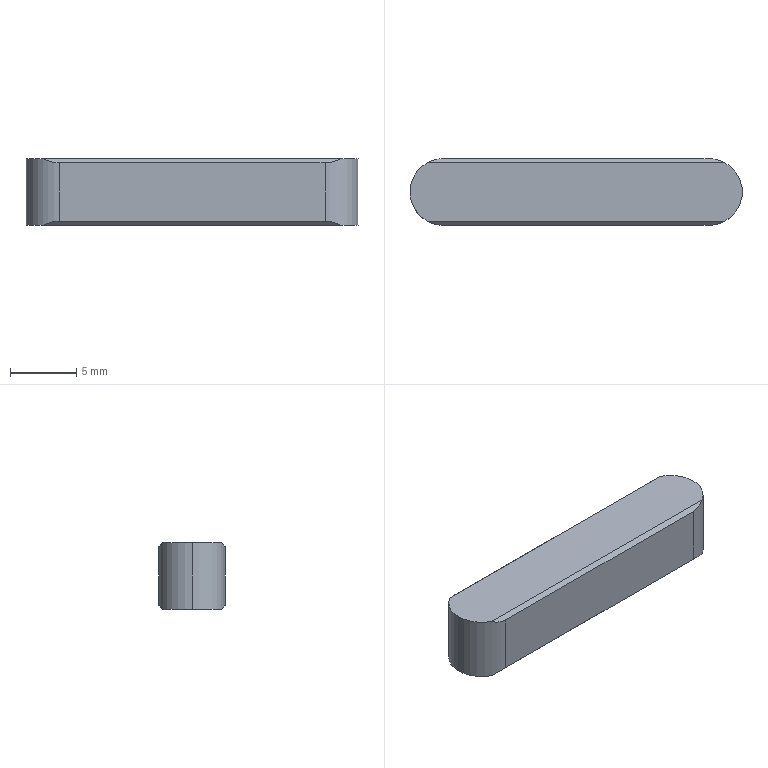Part | STEP file | 0228_010_KES5-25 | 1 solid | 11 faces | box 25 x 5 x 5 mm | volume 594.343 mm3 | plane 8 | cylinder 3 | commonest cylinder face diameters 5 x3
STEP:
#1=CARTESIAN_POINT('',(0.,0.,0.));
#2=DIRECTION('',(0.,0.,1.));
#3=DIRECTION('',(1.,0.,0.));
#4=AXIS2_PLACEMENT_3D('',#1,#2,#3);
#5=CARTESIAN_POINT('',(1.313,0.3,5.));
#6=VERTEX_POINT('',#5);
#7=CARTESIAN_POINT('',(0.,2.5,5.));
#8=VERTEX_POINT('',#7);
#9=CARTESIAN_POINT('',(2.5,2.5,5.));
#10=DIRECTION('',(0.,0.,-1.));
#11=DIRECTION('',(-1.,0.,0.));
#12=AXIS2_PLACEMENT_3D('',#9,#10,#11);
#13=CIRCLE('',#12,2.5);
#14=CARTESIAN_POINT('',(2.5,2.5,0.));
#15=DIRECTION('',(0.,0.,-1.));
#16=DIRECTION('',(-1.,0.,0.));
#17=AXIS2_PLACEMENT_3D('',#14,#15,#16);
#18=CYLINDRICAL_SURFACE('',#17,2.5);
#19=CARTESIAN_POINT('',(0.,-5.));
#20=DIRECTION('',(1.,0.));
#21=VECTOR('',#20,1.);
#22=LINE('',#19,#21);
#23=(GEOMETRIC_REPRESENTATION_CONTEXT(2)PARAMETRIC_REPRESENTATION_CONTEXT()REPRESENTATION_CONTEXT('',''));
#24=DEFINITIONAL_REPRESENTATION('',(#22),#23);
#25=PCURVE('',#18,#24);
#26=CARTESIAN_POINT('',(0.,0.,5.));
#27=DIRECTION('',(0.,0.,1.));
#28=DIRECTION('',(1.,0.,0.));
#29=AXIS2_PLACEMENT_3D('',#26,#27,#28);
#30=PLANE('',#29);
#31=CARTESIAN_POINT('',(0.,2.5));
#32=CARTESIAN_POINT('',(0.,6.83));
#33=CARTESIAN_POINT('',(3.75,4.665));
#34=CARTESIAN_POINT('',(7.5,2.5));
#35=CARTESIAN_POINT('',(3.75,0.3349));
#36=CARTESIAN_POINT('',(0.,-1.83));
#37=CARTESIAN_POINT('',(0.,2.5));
#38=(BOUNDED_CURVE()B_SPLINE_CURVE(2,(#31,#32,#33,#34,#35,#36,#37),.UNSPECIFIED.,.T.,.F.)B_SPLINE_CURVE_WITH_KNOTS((1,2,2,2,2,1),(-2.094,0.,2.094,4.189,6.283,8.378),.UNSPECIFIED.)CURVE()GEOMETRIC_REPRESENTATION_ITEM()RATIONAL_B_SPLINE_CURVE((1.,0.5,1.,0.5,1.,0.5,1.))REPRESENTATION_ITEM(''));
#39=(GEOMETRIC_REPRESENTATION_CONTEXT(2)PARAMETRIC_REPRESENTATION_CONTEXT()REPRESENTATION_CONTEXT('',''));
#40=DEFINITIONAL_REPRESENTATION('',(#38),#39);
#41=PCURVE('',#30,#40);
#42=SURFACE_CURVE('',#13,(#25,#41),.PCURVE_S1.);
#43=EDGE_CURVE('',#6,#8,#42,.T.);
#44=ORIENTED_EDGE('',*,*,#43,.T.);
#45=CARTESIAN_POINT('',(0.,2.5,0.));
#46=VERTEX_POINT('',#45);
#47=CARTESIAN_POINT('',(0.,2.5,0.));
#48=DIRECTION('',(0.,0.,-1.));
#49=VECTOR('',#48,1.);
#50=LINE('',#47,#49);
#51=CARTESIAN_POINT('',(6.283,0.));
#52=DIRECTION('',(0.,1.));
#53=VECTOR('',#52,1.);
#54=LINE('',#51,#53);
#55=(GEOMETRIC_REPRESENTATION_CONTEXT(2)PARAMETRIC_REPRESENTATION_CONTEXT()REPRESENTATION_CONTEXT('',''));
#56=DEFINITIONAL_REPRESENTATION('',(#54),#55);
#57=PCURVE('',#18,#56);
#58=CARTESIAN_POINT('',(2.5,2.5,0.));
#59=DIRECTION('',(0.,0.,-1.));
#60=DIRECTION('',(-1.,0.,0.));
#61=AXIS2_PLACEMENT_3D('',#58,#59,#60);
#62=CYLINDRICAL_SURFACE('',#61,2.5);
#63=CARTESIAN_POINT('',(0.,0.));
#64=DIRECTION('',(0.,1.));
#65=VECTOR('',#64,1.);
#66=LINE('',#63,#65);
#67=(GEOMETRIC_REPRESENTATION_CONTEXT(2)PARAMETRIC_REPRESENTATION_CONTEXT()REPRESENTATION_CONTEXT('',''));
#68=DEFINITIONAL_REPRESENTATION('',(#66),#67);
#69=PCURVE('',#62,#68);
#70=SURFACE_CURVE('',#50,(#57,#69),.PCURVE_S1.);
#71=EDGE_CURVE('',#8,#46,#70,.T.);
#72=ORIENTED_EDGE('',*,*,#71,.T.);
#73=CARTESIAN_POINT('',(1.313,0.3,0.));
#74=VERTEX_POINT('',#73);
#75=CARTESIAN_POINT('',(2.5,2.5,0.));
#76=DIRECTION('',(0.,0.,1.));
#77=DIRECTION('',(-1.,0.,0.));
#78=AXIS2_PLACEMENT_3D('',#75,#76,#77);
#79=CIRCLE('',#78,2.5);
#80=CARTESIAN_POINT('',(6.283,0.));
#81=DIRECTION('',(-1.,0.));
#82=VECTOR('',#81,1.);
#83=LINE('',#80,#82);
#84=(GEOMETRIC_REPRESENTATION_CONTEXT(2)PARAMETRIC_REPRESENTATION_CONTEXT()REPRESENTATION_CONTEXT('',''));
#85=DEFINITIONAL_REPRESENTATION('',(#83),#84);
#86=PCURVE('',#18,#85);
#87=CARTESIAN_POINT('',(0.,0.,0.));
#88=DIRECTION('',(0.,0.,1.));
#89=DIRECTION('',(1.,0.,0.));
#90=AXIS2_PLACEMENT_3D('',#87,#88,#89);
#91=PLANE('',#90);
#92=CARTESIAN_POINT('',(2.5,2.5));
#93=DIRECTION('',(-1.,0.));
#94=AXIS2_PLACEMENT_2D('',#92,#93);
#95=CIRCLE('',#94,2.5);
#96=(GEOMETRIC_REPRESENTATION_CONTEXT(2)PARAMETRIC_REPRESENTATION_CONTEXT()REPRESENTATION_CONTEXT('',''));
#97=DEFINITIONAL_REPRESENTATION('',(#95),#96);
#98=PCURVE('',#91,#97);
#99=SURFACE_CURVE('',#79,(#86,#98),.PCURVE_S1.);
#100=EDGE_CURVE('',#46,#74,#99,.T.);
#101=ORIENTED_EDGE('',*,*,#100,.T.);
#102=CARTESIAN_POINT('',(2.5,0.,0.3));
#103=VERTEX_POINT('',#102);
#104=CARTESIAN_POINT('',(1.313,0.3,0.));
#105=CARTESIAN_POINT('',(1.679,0.1021,0.1979));
#106=CARTESIAN_POINT('',(2.083,0.,0.3));
#107=CARTESIAN_POINT('',(2.5,0.,0.3));
#108=(BOUNDED_CURVE()B_SPLINE_CURVE(3,(#104,#105,#106,#107),.UNSPECIFIED.,.F.,.F.)B_SPLINE_CURVE_WITH_KNOTS((4,4),(2.647,3.142),.PIECEWISE_BEZIER_KNOTS.)CURVE()GEOMETRIC_REPRESENTATION_ITEM()RATIONAL_B_SPLINE_CURVE((1.,0.9797,0.9797,1.))REPRESENTATION_ITEM(''));
#109=CARTESIAN_POINT('',(5.207,0.));
#110=CARTESIAN_POINT('',(5.2,-0.008814));
#111=CARTESIAN_POINT('',(5.185,-0.0261));
#112=CARTESIAN_POINT('',(5.163,-0.05099));
#113=CARTESIAN_POINT('',(5.14,-0.07481));
#114=CARTESIAN_POINT('',(5.118,-0.09752));
#115=CARTESIAN_POINT('',(5.095,-0.1191));
#116=CARTESIAN_POINT('',(5.073,-0.1396));
#117=CARTESIAN_POINT('',(5.05,-0.1589));
#118=CARTESIAN_POINT('',(5.028,-0.177));
#119=CARTESIAN_POINT('',(5.005,-0.1939));
#120=CARTESIAN_POINT('',(4.982,-0.2096));
#121=CARTESIAN_POINT('',(4.96,-0.224));
#122=CARTESIAN_POINT('',(4.937,-0.2373));
#123=CARTESIAN_POINT('',(4.915,-0.2493));
#124=CARTESIAN_POINT('',(4.892,-0.26));
#125=CARTESIAN_POINT('',(4.869,-0.2694));
#126=CARTESIAN_POINT('',(4.847,-0.2776));
#127=CARTESIAN_POINT('',(4.824,-0.2845));
#128=CARTESIAN_POINT('',(4.802,-0.2902));
#129=CARTESIAN_POINT('',(4.779,-0.2946));
#130=CARTESIAN_POINT('',(4.757,-0.2977));
#131=CARTESIAN_POINT('',(4.735,-0.2996));
#132=CARTESIAN_POINT('',(4.72,-0.3));
#133=CARTESIAN_POINT('',(4.712,-0.3));
#134=B_SPLINE_CURVE_WITH_KNOTS('',3,(#109,#110,#111,#112,#113,#114,#115,#116,#117,#118,#119,#120,#121,#122,#123,#124,#125,#126,#127,#128,#129,#130,#131,#132,#133),.UNSPECIFIED.,.F.,.F.,(4,1,1,1,1,1,1,1,1,1,1,1,1,1,1,1,1,1,1,1,1,1,4),(2.647,2.669,2.692,2.714,2.737,2.759,2.782,2.804,2.827,2.849,2.872,2.894,2.917,2.939,2.962,2.984,3.007,3.029,3.052,3.074,3.097,3.119,3.142),.QUASI_UNIFORM_KNOTS.);
#135=(GEOMETRIC_REPRESENTATION_CONTEXT(2)PARAMETRIC_REPRESENTATION_CONTEXT()REPRESENTATION_CONTEXT('',''));
#136=DEFINITIONAL_REPRESENTATION('',(#134),#135);
#137=PCURVE('',#18,#136);
#138=CARTESIAN_POINT('',(0.,0.,0.3));
#139=DIRECTION('',(0.,0.7071,0.7071));
#140=DIRECTION('',(0.,-0.7071,0.7071));
#141=AXIS2_PLACEMENT_3D('',#138,#139,#140);
#142=PLANE('',#141);
#143=CARTESIAN_POINT('',(-0.4243,1.313));
#144=CARTESIAN_POINT('',(-0.1444,1.679));
#145=CARTESIAN_POINT('',(0.,2.083));
#146=CARTESIAN_POINT('',(0.,2.5));
#147=(BOUNDED_CURVE()B_SPLINE_CURVE(3,(#143,#144,#145,#146),.UNSPECIFIED.,.F.,.F.)B_SPLINE_CURVE_WITH_KNOTS((4,4),(2.647,3.142),.PIECEWISE_BEZIER_KNOTS.)CURVE()GEOMETRIC_REPRESENTATION_ITEM()RATIONAL_B_SPLINE_CURVE((1.,0.9797,0.9797,1.))REPRESENTATION_ITEM(''));
#148=(GEOMETRIC_REPRESENTATION_CONTEXT(2)PARAMETRIC_REPRESENTATION_CONTEXT()REPRESENTATION_CONTEXT('',''));
#149=DEFINITIONAL_REPRESENTATION('',(#147),#148);
#150=PCURVE('',#142,#149);
#151=SURFACE_CURVE('',#108,(#137,#150),.PCURVE_S1.);
#152=EDGE_CURVE('',#74,#103,#151,.T.);
#153=ORIENTED_EDGE('',*,*,#152,.T.);
#154=CARTESIAN_POINT('',(2.5,0.,4.7));
#155=VERTEX_POINT('',#154);
#156=CARTESIAN_POINT('',(2.5,0.,0.));
#157=DIRECTION('',(0.,0.,1.));
#158=VECTOR('',#157,1.);
#159=LINE('',#156,#158);
#160=CARTESIAN_POINT('',(4.712,0.));
#161=DIRECTION('',(0.,-1.));
#162=VECTOR('',#161,1.);
#163=LINE('',#160,#162);
#164=(GEOMETRIC_REPRESENTATION_CONTEXT(2)PARAMETRIC_REPRESENTATION_CONTEXT()REPRESENTATION_CONTEXT('',''));
#165=DEFINITIONAL_REPRESENTATION('',(#163),#164);
#166=PCURVE('',#18,#165);
#167=CARTESIAN_POINT('',(22.5,0.,0.));
#168=DIRECTION('',(0.,-1.,0.));
#169=DIRECTION('',(0.,0.,-1.));
#170=AXIS2_PLACEMENT_3D('',#167,#168,#169);
#171=PLANE('',#170);
#172=CARTESIAN_POINT('',(0.,-20.));
#173=DIRECTION('',(-1.,0.));
#174=VECTOR('',#173,1.);
#175=LINE('',#172,#174);
#176=(GEOMETRIC_REPRESENTATION_CONTEXT(2)PARAMETRIC_REPRESENTATION_CONTEXT()REPRESENTATION_CONTEXT('',''));
#177=DEFINITIONAL_REPRESENTATION('',(#175),#176);
#178=PCURVE('',#171,#177);
#179=SURFACE_CURVE('',#159,(#166,#178),.PCURVE_S1.);
#180=EDGE_CURVE('',#103,#155,#179,.T.);
#181=ORIENTED_EDGE('',*,*,#180,.T.);
#182=CARTESIAN_POINT('',(2.5,0.,4.7));
#183=CARTESIAN_POINT('',(2.083,0.,4.7));
#184=CARTESIAN_POINT('',(1.679,0.1021,4.802));
#185=CARTESIAN_POINT('',(1.313,0.3,5.));
#186=(BOUNDED_CURVE()B_SPLINE_CURVE(3,(#182,#183,#184,#185),.UNSPECIFIED.,.F.,.F.)B_SPLINE_CURVE_WITH_KNOTS((4,4),(0.,0.4949),.PIECEWISE_BEZIER_KNOTS.)CURVE()GEOMETRIC_REPRESENTATION_ITEM()RATIONAL_B_SPLINE_CURVE((1.,0.9797,0.9797,1.))REPRESENTATION_ITEM(''));
#187=CARTESIAN_POINT('',(4.712,-4.7));
#188=CARTESIAN_POINT('',(4.72,-4.7));
#189=CARTESIAN_POINT('',(4.735,-4.7));
#190=CARTESIAN_POINT('',(4.757,-4.702));
#191=CARTESIAN_POINT('',(4.779,-4.705));
#192=CARTESIAN_POINT('',(4.802,-4.71));
#193=CARTESIAN_POINT('',(4.824,-4.715));
#194=CARTESIAN_POINT('',(4.847,-4.722));
#195=CARTESIAN_POINT('',(4.869,-4.731));
#196=CARTESIAN_POINT('',(4.892,-4.74));
#197=CARTESIAN_POINT('',(4.915,-4.751));
#198=CARTESIAN_POINT('',(4.937,-4.763));
#199=CARTESIAN_POINT('',(4.96,-4.776));
#200=CARTESIAN_POINT('',(4.982,-4.79));
#201=CARTESIAN_POINT('',(5.005,-4.806));
#202=CARTESIAN_POINT('',(5.028,-4.823));
#203=CARTESIAN_POINT('',(5.05,-4.841));
#204=CARTESIAN_POINT('',(5.073,-4.86));
#205=CARTESIAN_POINT('',(5.095,-4.881));
#206=CARTESIAN_POINT('',(5.118,-4.902));
#207=CARTESIAN_POINT('',(5.14,-4.925));
#208=CARTESIAN_POINT('',(5.163,-4.949));
#209=CARTESIAN_POINT('',(5.185,-4.974));
#210=CARTESIAN_POINT('',(5.2,-4.991));
#211=CARTESIAN_POINT('',(5.207,-5.));
#212=B_SPLINE_CURVE_WITH_KNOTS('',3,(#187,#188,#189,#190,#191,#192,#193,#194,#195,#196,#197,#198,#199,#200,#201,#202,#203,#204,#205,#206,#207,#208,#209,#210,#211),.UNSPECIFIED.,.F.,.F.,(4,1,1,1,1,1,1,1,1,1,1,1,1,1,1,1,1,1,1,1,1,1,4),(0.,0.0225,0.04499,0.06749,0.08999,0.1125,0.135,0.1575,0.18,0.2025,0.225,0.2475,0.27,0.2925,0.315,0.3375,0.36,0.3824,0.4049,0.4274,0.4499,0.4724,0.4949),.QUASI_UNIFORM_KNOTS.);
#213=(GEOMETRIC_REPRESENTATION_CONTEXT(2)PARAMETRIC_REPRESENTATION_CONTEXT()REPRESENTATION_CONTEXT('',''));
#214=DEFINITIONAL_REPRESENTATION('',(#212),#213);
#215=PCURVE('',#18,#214);
#216=CARTESIAN_POINT('',(0.,0.3,5.));
#217=DIRECTION('',(0.,0.7071,-0.7071));
#218=DIRECTION('',(0.,0.7071,0.7071));
#219=AXIS2_PLACEMENT_3D('',#216,#217,#218);
#220=PLANE('',#219);
#221=CARTESIAN_POINT('',(-0.4243,2.5));
#222=CARTESIAN_POINT('',(-0.4243,2.083));
#223=CARTESIAN_POINT('',(-0.2799,1.679));
#224=CARTESIAN_POINT('',(0.,1.313));
#225=(BOUNDED_CURVE()B_SPLINE_CURVE(3,(#221,#222,#223,#224),.UNSPECIFIED.,.F.,.F.)B_SPLINE_CURVE_WITH_KNOTS((4,4),(0.,0.4949),.PIECEWISE_BEZIER_KNOTS.)CURVE()GEOMETRIC_REPRESENTATION_ITEM()RATIONAL_B_SPLINE_CURVE((1.,0.9797,0.9797,1.))REPRESENTATION_ITEM(''));
#226=(GEOMETRIC_REPRESENTATION_CONTEXT(2)PARAMETRIC_REPRESENTATION_CONTEXT()REPRESENTATION_CONTEXT('',''));
#227=DEFINITIONAL_REPRESENTATION('',(#225),#226);
#228=PCURVE('',#220,#227);
#229=SURFACE_CURVE('',#186,(#215,#228),.PCURVE_S1.);
#230=EDGE_CURVE('',#155,#6,#229,.T.);
#231=ORIENTED_EDGE('',*,*,#230,.T.);
#232=EDGE_LOOP('',(#44,#72,#101,#153,#181,#231));
#233=FACE_BOUND('',#232,.T.);
#234=ADVANCED_FACE('',(#233),#18,.T.);
#235=CARTESIAN_POINT('',(1.313,4.7,0.));
#236=VERTEX_POINT('',#235);
#237=CARTESIAN_POINT('',(2.5,2.5,0.));
#238=DIRECTION('',(0.,0.,1.));
#239=DIRECTION('',(-1.,0.,0.));
#240=AXIS2_PLACEMENT_3D('',#237,#238,#239);
#241=CIRCLE('',#240,2.5);
#242=CARTESIAN_POINT('',(2.5,2.5));
#243=DIRECTION('',(-1.,0.));
#244=AXIS2_PLACEMENT_2D('',#242,#243);
#245=CIRCLE('',#244,2.5);
#246=(GEOMETRIC_REPRESENTATION_CONTEXT(2)PARAMETRIC_REPRESENTATION_CONTEXT()REPRESENTATION_CONTEXT('',''));
#247=DEFINITIONAL_REPRESENTATION('',(#245),#246);
#248=PCURVE('',#91,#247);
#249=CARTESIAN_POINT('',(6.283,0.));
#250=DIRECTION('',(-1.,0.));
#251=VECTOR('',#250,1.);
#252=LINE('',#249,#251);
#253=(GEOMETRIC_REPRESENTATION_CONTEXT(2)PARAMETRIC_REPRESENTATION_CONTEXT()REPRESENTATION_CONTEXT('',''));
#254=DEFINITIONAL_REPRESENTATION('',(#252),#253);
#255=PCURVE('',#62,#254);
#256=SURFACE_CURVE('',#241,(#248,#255),.PCURVE_S1.);
#257=EDGE_CURVE('',#236,#46,#256,.T.);
#258=ORIENTED_EDGE('',*,*,#257,.F.);
#259=CARTESIAN_POINT('',(23.687,4.7,0.));
#260=VERTEX_POINT('',#259);
#261=CARTESIAN_POINT('',(0.,4.7,0.));
#262=DIRECTION('',(-1.,0.,0.));
#263=VECTOR('',#262,1.);
#264=LINE('',#261,#263);
#265=CARTESIAN_POINT('',(0.,4.7));
#266=DIRECTION('',(-1.,0.));
#267=VECTOR('',#266,1.);
#268=LINE('',#265,#267);
#269=(GEOMETRIC_REPRESENTATION_CONTEXT(2)PARAMETRIC_REPRESENTATION_CONTEXT()REPRESENTATION_CONTEXT('',''));
#270=DEFINITIONAL_REPRESENTATION('',(#268),#269);
#271=PCURVE('',#91,#270);
#272=CARTESIAN_POINT('',(0.,4.7,0.));
#273=DIRECTION('',(0.,-0.7071,0.7071));
#274=DIRECTION('',(0.,-0.7071,-0.7071));
#275=AXIS2_PLACEMENT_3D('',#272,#273,#274);
#276=PLANE('',#275);
#277=CARTESIAN_POINT('',(0.,0.));
#278=DIRECTION('',(0.,-1.));
#279=VECTOR('',#278,1.);
#280=LINE('',#277,#279);
#281=(GEOMETRIC_REPRESENTATION_CONTEXT(2)PARAMETRIC_REPRESENTATION_CONTEXT()REPRESENTATION_CONTEXT('',''));
#282=DEFINITIONAL_REPRESENTATION('',(#280),#281);
#283=PCURVE('',#276,#282);
#284=SURFACE_CURVE('',#264,(#271,#283),.PCURVE_S1.);
#285=EDGE_CURVE('',#260,#236,#284,.T.);
#286=ORIENTED_EDGE('',*,*,#285,.F.);
#287=CARTESIAN_POINT('',(23.687,0.3,0.));
#288=VERTEX_POINT('',#287);
#289=CARTESIAN_POINT('',(22.5,2.5,0.));
#290=DIRECTION('',(0.,0.,1.));
#291=DIRECTION('',(-1.,0.,0.));
#292=AXIS2_PLACEMENT_3D('',#289,#290,#291);
#293=CIRCLE('',#292,2.5);
#294=CARTESIAN_POINT('',(22.5,2.5));
#295=DIRECTION('',(-1.,0.));
#296=AXIS2_PLACEMENT_2D('',#294,#295);
#297=CIRCLE('',#296,2.5);
#298=(GEOMETRIC_REPRESENTATION_CONTEXT(2)PARAMETRIC_REPRESENTATION_CONTEXT()REPRESENTATION_CONTEXT('',''));
#299=DEFINITIONAL_REPRESENTATION('',(#297),#298);
#300=PCURVE('',#91,#299);
#301=CARTESIAN_POINT('',(22.5,2.5,0.));
#302=DIRECTION('',(0.,0.,-1.));
#303=DIRECTION('',(-1.,0.,0.));
#304=AXIS2_PLACEMENT_3D('',#301,#302,#303);
#305=CYLINDRICAL_SURFACE('',#304,2.5);
#306=CARTESIAN_POINT('',(6.283,0.));
#307=DIRECTION('',(-1.,0.));
#308=VECTOR('',#307,1.);
#309=LINE('',#306,#308);
#310=(GEOMETRIC_REPRESENTATION_CONTEXT(2)PARAMETRIC_REPRESENTATION_CONTEXT()REPRESENTATION_CONTEXT('',''));
#311=DEFINITIONAL_REPRESENTATION('',(#309),#310);
#312=PCURVE('',#305,#311);
#313=SURFACE_CURVE('',#293,(#300,#312),.PCURVE_S1.);
#314=EDGE_CURVE('',#288,#260,#313,.T.);
#315=ORIENTED_EDGE('',*,*,#314,.F.);
#316=CARTESIAN_POINT('',(0.,0.3,0.));
#317=DIRECTION('',(1.,0.,0.));
#318=VECTOR('',#317,1.);
#319=LINE('',#316,#318);
#320=CARTESIAN_POINT('',(0.,0.3));
#321=DIRECTION('',(1.,0.));
#322=VECTOR('',#321,1.);
#323=LINE('',#320,#322);
#324=(GEOMETRIC_REPRESENTATION_CONTEXT(2)PARAMETRIC_REPRESENTATION_CONTEXT()REPRESENTATION_CONTEXT('',''));
#325=DEFINITIONAL_REPRESENTATION('',(#323),#324);
#326=PCURVE('',#91,#325);
#327=CARTESIAN_POINT('',(-0.4243,0.));
#328=DIRECTION('',(0.,1.));
#329=VECTOR('',#328,1.);
#330=LINE('',#327,#329);
#331=(GEOMETRIC_REPRESENTATION_CONTEXT(2)PARAMETRIC_REPRESENTATION_CONTEXT()REPRESENTATION_CONTEXT('',''));
#332=DEFINITIONAL_REPRESENTATION('',(#330),#331);
#333=PCURVE('',#142,#332);
#334=SURFACE_CURVE('',#319,(#326,#333),.PCURVE_S1.);
#335=EDGE_CURVE('',#74,#288,#334,.T.);
#336=ORIENTED_EDGE('',*,*,#335,.F.);
#337=ORIENTED_EDGE('',*,*,#100,.F.);
#338=EDGE_LOOP('',(#258,#286,#315,#336,#337));
#339=FACE_BOUND('',#338,.T.);
#340=ADVANCED_FACE('',(#339),#91,.F.);
#341=CARTESIAN_POINT('',(22.5,0.,0.3));
#342=VERTEX_POINT('',#341);
#343=CARTESIAN_POINT('',(0.,0.,0.3));
#344=DIRECTION('',(1.,0.,0.));
#345=VECTOR('',#344,1.);
#346=LINE('',#343,#345);
#347=CARTESIAN_POINT('',(0.,0.));
#348=DIRECTION('',(0.,1.));
#349=VECTOR('',#348,1.);
#350=LINE('',#347,#349);
#351=(GEOMETRIC_REPRESENTATION_CONTEXT(2)PARAMETRIC_REPRESENTATION_CONTEXT()REPRESENTATION_CONTEXT('',''));
#352=DEFINITIONAL_REPRESENTATION('',(#350),#351);
#353=PCURVE('',#142,#352);
#354=CARTESIAN_POINT('',(-0.3,-22.5));
#355=DIRECTION('',(0.,1.));
#356=VECTOR('',#355,1.);
#357=LINE('',#354,#356);
#358=(GEOMETRIC_REPRESENTATION_CONTEXT(2)PARAMETRIC_REPRESENTATION_CONTEXT()REPRESENTATION_CONTEXT('',''));
#359=DEFINITIONAL_REPRESENTATION('',(#357),#358);
#360=PCURVE('',#171,#359);
#361=SURFACE_CURVE('',#346,(#353,#360),.PCURVE_S1.);
#362=EDGE_CURVE('',#103,#342,#361,.T.);
#363=ORIENTED_EDGE('',*,*,#362,.F.);
#364=ORIENTED_EDGE('',*,*,#152,.F.);
#365=ORIENTED_EDGE('',*,*,#335,.T.);
#366=CARTESIAN_POINT('',(22.5,0.,0.3));
#367=CARTESIAN_POINT('',(22.917,0.,0.3));
#368=CARTESIAN_POINT('',(23.321,0.1021,0.1979));
#369=CARTESIAN_POINT('',(23.687,0.3,0.));
#370=(BOUNDED_CURVE()B_SPLINE_CURVE(3,(#366,#367,#368,#369),.UNSPECIFIED.,.F.,.F.)B_SPLINE_CURVE_WITH_KNOTS((4,4),(3.142,3.637),.PIECEWISE_BEZIER_KNOTS.)CURVE()GEOMETRIC_REPRESENTATION_ITEM()RATIONAL_B_SPLINE_CURVE((1.,0.9797,0.9797,1.))REPRESENTATION_ITEM(''));
#371=CARTESIAN_POINT('',(0.,22.5));
#372=CARTESIAN_POINT('',(0.,22.917));
#373=CARTESIAN_POINT('',(-0.1444,23.321));
#374=CARTESIAN_POINT('',(-0.4243,23.687));
#375=(BOUNDED_CURVE()B_SPLINE_CURVE(3,(#371,#372,#373,#374),.UNSPECIFIED.,.F.,.F.)B_SPLINE_CURVE_WITH_KNOTS((4,4),(3.142,3.637),.PIECEWISE_BEZIER_KNOTS.)CURVE()GEOMETRIC_REPRESENTATION_ITEM()RATIONAL_B_SPLINE_CURVE((1.,0.9797,0.9797,1.))REPRESENTATION_ITEM(''));
#376=(GEOMETRIC_REPRESENTATION_CONTEXT(2)PARAMETRIC_REPRESENTATION_CONTEXT()REPRESENTATION_CONTEXT('',''));
#377=DEFINITIONAL_REPRESENTATION('',(#375),#376);
#378=PCURVE('',#142,#377);
#379=CARTESIAN_POINT('',(4.712,-0.3));
#380=CARTESIAN_POINT('',(4.705,-0.3));
#381=CARTESIAN_POINT('',(4.69,-0.2996));
#382=CARTESIAN_POINT('',(4.668,-0.2977));
#383=CARTESIAN_POINT('',(4.645,-0.2946));
#384=CARTESIAN_POINT('',(4.623,-0.2902));
#385=CARTESIAN_POINT('',(4.6,-0.2845));
#386=CARTESIAN_POINT('',(4.578,-0.2776));
#387=CARTESIAN_POINT('',(4.555,-0.2694));
#388=CARTESIAN_POINT('',(4.533,-0.26));
#389=CARTESIAN_POINT('',(4.51,-0.2493));
#390=CARTESIAN_POINT('',(4.488,-0.2373));
#391=CARTESIAN_POINT('',(4.465,-0.224));
#392=CARTESIAN_POINT('',(4.442,-0.2096));
#393=CARTESIAN_POINT('',(4.42,-0.1939));
#394=CARTESIAN_POINT('',(4.397,-0.177));
#395=CARTESIAN_POINT('',(4.375,-0.1589));
#396=CARTESIAN_POINT('',(4.352,-0.1396));
#397=CARTESIAN_POINT('',(4.329,-0.1191));
#398=CARTESIAN_POINT('',(4.307,-0.09752));
#399=CARTESIAN_POINT('',(4.285,-0.07481));
#400=CARTESIAN_POINT('',(4.262,-0.05099));
#401=CARTESIAN_POINT('',(4.24,-0.0261));
#402=CARTESIAN_POINT('',(4.225,-0.008814));
#403=CARTESIAN_POINT('',(4.217,0.));
#404=B_SPLINE_CURVE_WITH_KNOTS('',3,(#379,#380,#381,#382,#383,#384,#385,#386,#387,#388,#389,#390,#391,#392,#393,#394,#395,#396,#397,#398,#399,#400,#401,#402,#403),.UNSPECIFIED.,.F.,.F.,(4,1,1,1,1,1,1,1,1,1,1,1,1,1,1,1,1,1,1,1,1,1,4),(3.142,3.164,3.187,3.209,3.232,3.254,3.277,3.299,3.322,3.344,3.367,3.389,3.412,3.434,3.457,3.479,3.502,3.524,3.547,3.569,3.592,3.614,3.637),.QUASI_UNIFORM_KNOTS.);
#405=(GEOMETRIC_REPRESENTATION_CONTEXT(2)PARAMETRIC_REPRESENTATION_CONTEXT()REPRESENTATION_CONTEXT('',''));
#406=DEFINITIONAL_REPRESENTATION('',(#404),#405);
#407=PCURVE('',#305,#406);
#408=SURFACE_CURVE('',#370,(#378,#407),.PCURVE_S1.);
#409=EDGE_CURVE('',#342,#288,#408,.T.);
#410=ORIENTED_EDGE('',*,*,#409,.F.);
#411=EDGE_LOOP('',(#363,#364,#365,#410));
#412=FACE_BOUND('',#411,.T.);
#413=ADVANCED_FACE('',(#412),#142,.F.);
#414=ORIENTED_EDGE('',*,*,#71,.F.);
#415=CARTESIAN_POINT('',(1.313,4.7,5.));
#416=VERTEX_POINT('',#415);
#417=CARTESIAN_POINT('',(2.5,2.5,5.));
#418=DIRECTION('',(0.,0.,-1.));
#419=DIRECTION('',(-1.,0.,0.));
#420=AXIS2_PLACEMENT_3D('',#417,#418,#419);
#421=CIRCLE('',#420,2.5);
#422=CARTESIAN_POINT('',(0.,-5.));
#423=DIRECTION('',(1.,0.));
#424=VECTOR('',#423,1.);
#425=LINE('',#422,#424);
#426=(GEOMETRIC_REPRESENTATION_CONTEXT(2)PARAMETRIC_REPRESENTATION_CONTEXT()REPRESENTATION_CONTEXT('',''));
#427=DEFINITIONAL_REPRESENTATION('',(#425),#426);
#428=PCURVE('',#62,#427);
#429=CARTESIAN_POINT('',(0.,2.5));
#430=CARTESIAN_POINT('',(0.,6.83));
#431=CARTESIAN_POINT('',(3.75,4.665));
#432=CARTESIAN_POINT('',(7.5,2.5));
#433=CARTESIAN_POINT('',(3.75,0.3349));
#434=CARTESIAN_POINT('',(0.,-1.83));
#435=CARTESIAN_POINT('',(0.,2.5));
#436=(BOUNDED_CURVE()B_SPLINE_CURVE(2,(#429,#430,#431,#432,#433,#434,#435),.UNSPECIFIED.,.T.,.F.)B_SPLINE_CURVE_WITH_KNOTS((1,2,2,2,2,1),(-2.094,0.,2.094,4.189,6.283,8.378),.UNSPECIFIED.)CURVE()GEOMETRIC_REPRESENTATION_ITEM()RATIONAL_B_SPLINE_CURVE((1.,0.5,1.,0.5,1.,0.5,1.))REPRESENTATION_ITEM(''));
#437=(GEOMETRIC_REPRESENTATION_CONTEXT(2)PARAMETRIC_REPRESENTATION_CONTEXT()REPRESENTATION_CONTEXT('',''));
#438=DEFINITIONAL_REPRESENTATION('',(#436),#437);
#439=PCURVE('',#30,#438);
#440=SURFACE_CURVE('',#421,(#428,#439),.PCURVE_S1.);
#441=EDGE_CURVE('',#8,#416,#440,.T.);
#442=ORIENTED_EDGE('',*,*,#441,.T.);
#443=CARTESIAN_POINT('',(2.5,5.,4.7));
#444=VERTEX_POINT('',#443);
#445=CARTESIAN_POINT('',(1.313,4.7,5.));
#446=CARTESIAN_POINT('',(1.679,4.898,4.802));
#447=CARTESIAN_POINT('',(2.083,5.,4.7));
#448=CARTESIAN_POINT('',(2.5,5.,4.7));
#449=(BOUNDED_CURVE()B_SPLINE_CURVE(3,(#445,#446,#447,#448),.UNSPECIFIED.,.F.,.F.)B_SPLINE_CURVE_WITH_KNOTS((4,4),(5.788,6.283),.PIECEWISE_BEZIER_KNOTS.)CURVE()GEOMETRIC_REPRESENTATION_ITEM()RATIONAL_B_SPLINE_CURVE((1.,0.9797,0.9797,1.))REPRESENTATION_ITEM(''));
#450=CARTESIAN_POINT('',(1.076,-5.));
#451=CARTESIAN_POINT('',(1.083,-4.991));
#452=CARTESIAN_POINT('',(1.098,-4.974));
#453=CARTESIAN_POINT('',(1.121,-4.949));
#454=CARTESIAN_POINT('',(1.143,-4.925));
#455=CARTESIAN_POINT('',(1.165,-4.902));
#456=CARTESIAN_POINT('',(1.188,-4.881));
#457=CARTESIAN_POINT('',(1.21,-4.86));
#458=CARTESIAN_POINT('',(1.233,-4.841));
#459=CARTESIAN_POINT('',(1.256,-4.823));
#460=CARTESIAN_POINT('',(1.278,-4.806));
#461=CARTESIAN_POINT('',(1.301,-4.79));
#462=CARTESIAN_POINT('',(1.323,-4.776));
#463=CARTESIAN_POINT('',(1.346,-4.763));
#464=CARTESIAN_POINT('',(1.369,-4.751));
#465=CARTESIAN_POINT('',(1.391,-4.74));
#466=CARTESIAN_POINT('',(1.414,-4.731));
#467=CARTESIAN_POINT('',(1.436,-4.722));
#468=CARTESIAN_POINT('',(1.459,-4.715));
#469=CARTESIAN_POINT('',(1.481,-4.71));
#470=CARTESIAN_POINT('',(1.504,-4.705));
#471=CARTESIAN_POINT('',(1.526,-4.702));
#472=CARTESIAN_POINT('',(1.549,-4.7));
#473=CARTESIAN_POINT('',(1.563,-4.7));
#474=CARTESIAN_POINT('',(1.571,-4.7));
#475=B_SPLINE_CURVE_WITH_KNOTS('',3,(#450,#451,#452,#453,#454,#455,#456,#457,#458,#459,#460,#461,#462,#463,#464,#465,#466,#467,#468,#469,#470,#471,#472,#473,#474),.UNSPECIFIED.,.F.,.F.,(4,1,1,1,1,1,1,1,1,1,1,1,1,1,1,1,1,1,1,1,1,1,4),(5.788,5.811,5.833,5.856,5.878,5.901,5.923,5.946,5.968,5.991,6.013,6.036,6.058,6.081,6.103,6.126,6.148,6.171,6.193,6.216,6.238,6.261,6.283),.QUASI_UNIFORM_KNOTS.);
#476=(GEOMETRIC_REPRESENTATION_CONTEXT(2)PARAMETRIC_REPRESENTATION_CONTEXT()REPRESENTATION_CONTEXT('',''));
#477=DEFINITIONAL_REPRESENTATION('',(#475),#476);
#478=PCURVE('',#62,#477);
#479=CARTESIAN_POINT('',(0.,5.,4.7));
#480=DIRECTION('',(0.,-0.7071,-0.7071));
#481=DIRECTION('',(0.,0.7071,-0.7071));
#482=AXIS2_PLACEMENT_3D('',#479,#480,#481);
#483=PLANE('',#482);
#484=CARTESIAN_POINT('',(-0.4243,1.313));
#485=CARTESIAN_POINT('',(-0.1444,1.679));
#486=CARTESIAN_POINT('',(0.,2.083));
#487=CARTESIAN_POINT('',(0.,2.5));
#488=(BOUNDED_CURVE()B_SPLINE_CURVE(3,(#484,#485,#486,#487),.UNSPECIFIED.,.F.,.F.)B_SPLINE_CURVE_WITH_KNOTS((4,4),(5.788,6.283),.PIECEWISE_BEZIER_KNOTS.)CURVE()GEOMETRIC_REPRESENTATION_ITEM()RATIONAL_B_SPLINE_CURVE((1.,0.9797,0.9797,1.))REPRESENTATION_ITEM(''));
#489=(GEOMETRIC_REPRESENTATION_CONTEXT(2)PARAMETRIC_REPRESENTATION_CONTEXT()REPRESENTATION_CONTEXT('',''));
#490=DEFINITIONAL_REPRESENTATION('',(#488),#489);
#491=PCURVE('',#483,#490);
#492=SURFACE_CURVE('',#449,(#478,#491),.PCURVE_S1.);
#493=EDGE_CURVE('',#416,#444,#492,.T.);
#494=ORIENTED_EDGE('',*,*,#493,.T.);
#495=CARTESIAN_POINT('',(2.5,5.,0.3));
#496=VERTEX_POINT('',#495);
#497=CARTESIAN_POINT('',(2.5,5.,0.));
#498=DIRECTION('',(0.,0.,-1.));
#499=VECTOR('',#498,1.);
#500=LINE('',#497,#499);
#501=CARTESIAN_POINT('',(1.571,0.));
#502=DIRECTION('',(0.,1.));
#503=VECTOR('',#502,1.);
#504=LINE('',#501,#503);
#505=(GEOMETRIC_REPRESENTATION_CONTEXT(2)PARAMETRIC_REPRESENTATION_CONTEXT()REPRESENTATION_CONTEXT('',''));
#506=DEFINITIONAL_REPRESENTATION('',(#504),#505);
#507=PCURVE('',#62,#506);
#508=CARTESIAN_POINT('',(2.5,5.,0.));
#509=DIRECTION('',(0.,1.,0.));
#510=DIRECTION('',(0.,0.,1.));
#511=AXIS2_PLACEMENT_3D('',#508,#509,#510);
#512=PLANE('',#511);
#513=CARTESIAN_POINT('',(0.,0.));
#514=DIRECTION('',(-1.,0.));
#515=VECTOR('',#514,1.);
#516=LINE('',#513,#515);
#517=(GEOMETRIC_REPRESENTATION_CONTEXT(2)PARAMETRIC_REPRESENTATION_CONTEXT()REPRESENTATION_CONTEXT('',''));
#518=DEFINITIONAL_REPRESENTATION('',(#516),#517);
#519=PCURVE('',#512,#518);
#520=SURFACE_CURVE('',#500,(#507,#519),.PCURVE_S1.);
#521=EDGE_CURVE('',#444,#496,#520,.T.);
#522=ORIENTED_EDGE('',*,*,#521,.T.);
#523=CARTESIAN_POINT('',(2.5,5.,0.3));
#524=CARTESIAN_POINT('',(2.083,5.,0.3));
#525=CARTESIAN_POINT('',(1.679,4.898,0.1979));
#526=CARTESIAN_POINT('',(1.313,4.7,0.));
#527=(BOUNDED_CURVE()B_SPLINE_CURVE(3,(#523,#524,#525,#526),.UNSPECIFIED.,.F.,.F.)B_SPLINE_CURVE_WITH_KNOTS((4,4),(3.142,3.637),.PIECEWISE_BEZIER_KNOTS.)CURVE()GEOMETRIC_REPRESENTATION_ITEM()RATIONAL_B_SPLINE_CURVE((1.,0.9797,0.9797,1.))REPRESENTATION_ITEM(''));
#528=CARTESIAN_POINT('',(1.571,-0.3));
#529=CARTESIAN_POINT('',(1.563,-0.3));
#530=CARTESIAN_POINT('',(1.549,-0.2996));
#531=CARTESIAN_POINT('',(1.526,-0.2977));
#532=CARTESIAN_POINT('',(1.504,-0.2946));
#533=CARTESIAN_POINT('',(1.481,-0.2902));
#534=CARTESIAN_POINT('',(1.459,-0.2845));
#535=CARTESIAN_POINT('',(1.436,-0.2776));
#536=CARTESIAN_POINT('',(1.414,-0.2694));
#537=CARTESIAN_POINT('',(1.391,-0.26));
#538=CARTESIAN_POINT('',(1.369,-0.2493));
#539=CARTESIAN_POINT('',(1.346,-0.2373));
#540=CARTESIAN_POINT('',(1.323,-0.224));
#541=CARTESIAN_POINT('',(1.301,-0.2096));
#542=CARTESIAN_POINT('',(1.278,-0.1939));
#543=CARTESIAN_POINT('',(1.256,-0.177));
#544=CARTESIAN_POINT('',(1.233,-0.1589));
#545=CARTESIAN_POINT('',(1.21,-0.1396));
#546=CARTESIAN_POINT('',(1.188,-0.1191));
#547=CARTESIAN_POINT('',(1.165,-0.09752));
#548=CARTESIAN_POINT('',(1.143,-0.07481));
#549=CARTESIAN_POINT('',(1.121,-0.05099));
#550=CARTESIAN_POINT('',(1.098,-0.0261));
#551=CARTESIAN_POINT('',(1.083,-0.008814));
#552=CARTESIAN_POINT('',(1.076,0.));
#553=B_SPLINE_CURVE_WITH_KNOTS('',3,(#528,#529,#530,#531,#532,#533,#534,#535,#536,#537,#538,#539,#540,#541,#542,#543,#544,#545,#546,#547,#548,#549,#550,#551,#552),.UNSPECIFIED.,.F.,.F.,(4,1,1,1,1,1,1,1,1,1,1,1,1,1,1,1,1,1,1,1,1,1,4),(3.142,3.164,3.187,3.209,3.232,3.254,3.277,3.299,3.322,3.344,3.367,3.389,3.412,3.434,3.457,3.479,3.502,3.524,3.547,3.569,3.592,3.614,3.637),.QUASI_UNIFORM_KNOTS.);
#554=(GEOMETRIC_REPRESENTATION_CONTEXT(2)PARAMETRIC_REPRESENTATION_CONTEXT()REPRESENTATION_CONTEXT('',''));
#555=DEFINITIONAL_REPRESENTATION('',(#553),#554);
#556=PCURVE('',#62,#555);
#557=CARTESIAN_POINT('',(-0.4243,2.5));
#558=CARTESIAN_POINT('',(-0.4243,2.083));
#559=CARTESIAN_POINT('',(-0.2799,1.679));
#560=CARTESIAN_POINT('',(0.,1.313));
#561=(BOUNDED_CURVE()B_SPLINE_CURVE(3,(#557,#558,#559,#560),.UNSPECIFIED.,.F.,.F.)B_SPLINE_CURVE_WITH_KNOTS((4,4),(3.142,3.637),.PIECEWISE_BEZIER_KNOTS.)CURVE()GEOMETRIC_REPRESENTATION_ITEM()RATIONAL_B_SPLINE_CURVE((1.,0.9797,0.9797,1.))REPRESENTATION_ITEM(''));
#562=(GEOMETRIC_REPRESENTATION_CONTEXT(2)PARAMETRIC_REPRESENTATION_CONTEXT()REPRESENTATION_CONTEXT('',''));
#563=DEFINITIONAL_REPRESENTATION('',(#561),#562);
#564=PCURVE('',#276,#563);
#565=SURFACE_CURVE('',#527,(#556,#564),.PCURVE_S1.);
#566=EDGE_CURVE('',#496,#236,#565,.T.);
#567=ORIENTED_EDGE('',*,*,#566,.T.);
#568=ORIENTED_EDGE('',*,*,#257,.T.);
#569=EDGE_LOOP('',(#414,#442,#494,#522,#567,#568));
#570=FACE_BOUND('',#569,.T.);
#571=ADVANCED_FACE('',(#570),#62,.T.);
#572=ORIENTED_EDGE('',*,*,#285,.T.);
#573=ORIENTED_EDGE('',*,*,#566,.F.);
#574=CARTESIAN_POINT('',(22.5,5.,0.3));
#575=VERTEX_POINT('',#574);
#576=CARTESIAN_POINT('',(0.,5.,0.3));
#577=DIRECTION('',(-1.,0.,0.));
#578=VECTOR('',#577,1.);
#579=LINE('',#576,#578);
#580=CARTESIAN_POINT('',(-0.4243,0.));
#581=DIRECTION('',(0.,-1.));
#582=VECTOR('',#581,1.);
#583=LINE('',#580,#582);
#584=(GEOMETRIC_REPRESENTATION_CONTEXT(2)PARAMETRIC_REPRESENTATION_CONTEXT()REPRESENTATION_CONTEXT('',''));
#585=DEFINITIONAL_REPRESENTATION('',(#583),#584);
#586=PCURVE('',#276,#585);
#587=CARTESIAN_POINT('',(0.3,-2.5));
#588=DIRECTION('',(0.,-1.));
#589=VECTOR('',#588,1.);
#590=LINE('',#587,#589);
#591=(GEOMETRIC_REPRESENTATION_CONTEXT(2)PARAMETRIC_REPRESENTATION_CONTEXT()REPRESENTATION_CONTEXT('',''));
#592=DEFINITIONAL_REPRESENTATION('',(#590),#591);
#593=PCURVE('',#512,#592);
#594=SURFACE_CURVE('',#579,(#586,#593),.PCURVE_S1.);
#595=EDGE_CURVE('',#575,#496,#594,.T.);
#596=ORIENTED_EDGE('',*,*,#595,.F.);
#597=CARTESIAN_POINT('',(23.687,4.7,0.));
#598=CARTESIAN_POINT('',(23.321,4.898,0.1979));
#599=CARTESIAN_POINT('',(22.917,5.,0.3));
#600=CARTESIAN_POINT('',(22.5,5.,0.3));
#601=(BOUNDED_CURVE()B_SPLINE_CURVE(3,(#597,#598,#599,#600),.UNSPECIFIED.,.F.,.F.)B_SPLINE_CURVE_WITH_KNOTS((4,4),(2.647,3.142),.PIECEWISE_BEZIER_KNOTS.)CURVE()GEOMETRIC_REPRESENTATION_ITEM()RATIONAL_B_SPLINE_CURVE((1.,0.9797,0.9797,1.))REPRESENTATION_ITEM(''));
#602=CARTESIAN_POINT('',(0.,23.687));
#603=CARTESIAN_POINT('',(-0.2799,23.321));
#604=CARTESIAN_POINT('',(-0.4243,22.917));
#605=CARTESIAN_POINT('',(-0.4243,22.5));
#606=(BOUNDED_CURVE()B_SPLINE_CURVE(3,(#602,#603,#604,#605),.UNSPECIFIED.,.F.,.F.)B_SPLINE_CURVE_WITH_KNOTS((4,4),(2.647,3.142),.PIECEWISE_BEZIER_KNOTS.)CURVE()GEOMETRIC_REPRESENTATION_ITEM()RATIONAL_B_SPLINE_CURVE((1.,0.9797,0.9797,1.))REPRESENTATION_ITEM(''));
#607=(GEOMETRIC_REPRESENTATION_CONTEXT(2)PARAMETRIC_REPRESENTATION_CONTEXT()REPRESENTATION_CONTEXT('',''));
#608=DEFINITIONAL_REPRESENTATION('',(#606),#607);
#609=PCURVE('',#276,#608);
#610=CARTESIAN_POINT('',(2.066,0.));
#611=CARTESIAN_POINT('',(2.058,-0.008814));
#612=CARTESIAN_POINT('',(2.043,-0.0261));
#613=CARTESIAN_POINT('',(2.021,-0.05099));
#614=CARTESIAN_POINT('',(1.999,-0.07481));
#615=CARTESIAN_POINT('',(1.976,-0.09752));
#616=CARTESIAN_POINT('',(1.954,-0.1191));
#617=CARTESIAN_POINT('',(1.931,-0.1396));
#618=CARTESIAN_POINT('',(1.909,-0.1589));
#619=CARTESIAN_POINT('',(1.886,-0.177));
#620=CARTESIAN_POINT('',(1.863,-0.1939));
#621=CARTESIAN_POINT('',(1.841,-0.2096));
#622=CARTESIAN_POINT('',(1.818,-0.224));
#623=CARTESIAN_POINT('',(1.796,-0.2373));
#624=CARTESIAN_POINT('',(1.773,-0.2493));
#625=CARTESIAN_POINT('',(1.75,-0.26));
#626=CARTESIAN_POINT('',(1.728,-0.2694));
#627=CARTESIAN_POINT('',(1.705,-0.2776));
#628=CARTESIAN_POINT('',(1.683,-0.2845));
#629=CARTESIAN_POINT('',(1.66,-0.2902));
#630=CARTESIAN_POINT('',(1.638,-0.2946));
#631=CARTESIAN_POINT('',(1.615,-0.2977));
#632=CARTESIAN_POINT('',(1.593,-0.2996));
#633=CARTESIAN_POINT('',(1.578,-0.3));
#634=CARTESIAN_POINT('',(1.571,-0.3));
#635=B_SPLINE_CURVE_WITH_KNOTS('',3,(#610,#611,#612,#613,#614,#615,#616,#617,#618,#619,#620,#621,#622,#623,#624,#625,#626,#627,#628,#629,#630,#631,#632,#633,#634),.UNSPECIFIED.,.F.,.F.,(4,1,1,1,1,1,1,1,1,1,1,1,1,1,1,1,1,1,1,1,1,1,4),(2.647,2.669,2.692,2.714,2.737,2.759,2.782,2.804,2.827,2.849,2.872,2.894,2.917,2.939,2.962,2.984,3.007,3.029,3.052,3.074,3.097,3.119,3.142),.QUASI_UNIFORM_KNOTS.);
#636=(GEOMETRIC_REPRESENTATION_CONTEXT(2)PARAMETRIC_REPRESENTATION_CONTEXT()REPRESENTATION_CONTEXT('',''));
#637=DEFINITIONAL_REPRESENTATION('',(#635),#636);
#638=PCURVE('',#305,#637);
#639=SURFACE_CURVE('',#601,(#609,#638),.PCURVE_S1.);
#640=EDGE_CURVE('',#260,#575,#639,.T.);
#641=ORIENTED_EDGE('',*,*,#640,.F.);
#642=EDGE_LOOP('',(#572,#573,#596,#641));
#643=FACE_BOUND('',#642,.T.);
#644=ADVANCED_FACE('',(#643),#276,.F.);
#645=CARTESIAN_POINT('',(22.5,5.,4.7));
#646=VERTEX_POINT('',#645);
#647=CARTESIAN_POINT('',(23.687,4.7,5.));
#648=VERTEX_POINT('',#647);
#649=CARTESIAN_POINT('',(22.5,5.,4.7));
#650=CARTESIAN_POINT('',(22.917,5.,4.7));
#651=CARTESIAN_POINT('',(23.321,4.898,4.802));
#652=CARTESIAN_POINT('',(23.687,4.7,5.));
#653=(BOUNDED_CURVE()B_SPLINE_CURVE(3,(#649,#650,#651,#652),.UNSPECIFIED.,.F.,.F.)B_SPLINE_CURVE_WITH_KNOTS((4,4),(0.,0.4949),.PIECEWISE_BEZIER_KNOTS.)CURVE()GEOMETRIC_REPRESENTATION_ITEM()RATIONAL_B_SPLINE_CURVE((1.,0.9797,0.9797,1.))REPRESENTATION_ITEM(''));
#654=CARTESIAN_POINT('',(1.571,-4.7));
#655=CARTESIAN_POINT('',(1.578,-4.7));
#656=CARTESIAN_POINT('',(1.593,-4.7));
#657=CARTESIAN_POINT('',(1.615,-4.702));
#658=CARTESIAN_POINT('',(1.638,-4.705));
#659=CARTESIAN_POINT('',(1.66,-4.71));
#660=CARTESIAN_POINT('',(1.683,-4.715));
#661=CARTESIAN_POINT('',(1.705,-4.722));
#662=CARTESIAN_POINT('',(1.728,-4.731));
#663=CARTESIAN_POINT('',(1.75,-4.74));
#664=CARTESIAN_POINT('',(1.773,-4.751));
#665=CARTESIAN_POINT('',(1.796,-4.763));
#666=CARTESIAN_POINT('',(1.818,-4.776));
#667=CARTESIAN_POINT('',(1.841,-4.79));
#668=CARTESIAN_POINT('',(1.863,-4.806));
#669=CARTESIAN_POINT('',(1.886,-4.823));
#670=CARTESIAN_POINT('',(1.909,-4.841));
#671=CARTESIAN_POINT('',(1.931,-4.86));
#672=CARTESIAN_POINT('',(1.954,-4.881));
#673=CARTESIAN_POINT('',(1.976,-4.902));
#674=CARTESIAN_POINT('',(1.999,-4.925));
#675=CARTESIAN_POINT('',(2.021,-4.949));
#676=CARTESIAN_POINT('',(2.043,-4.974));
#677=CARTESIAN_POINT('',(2.058,-4.991));
#678=CARTESIAN_POINT('',(2.066,-5.));
#679=B_SPLINE_CURVE_WITH_KNOTS('',3,(#654,#655,#656,#657,#658,#659,#660,#661,#662,#663,#664,#665,#666,#667,#668,#669,#670,#671,#672,#673,#674,#675,#676,#677,#678),.UNSPECIFIED.,.F.,.F.,(4,1,1,1,1,1,1,1,1,1,1,1,1,1,1,1,1,1,1,1,1,1,4),(0.,0.0225,0.04499,0.06749,0.08999,0.1125,0.135,0.1575,0.18,0.2025,0.225,0.2475,0.27,0.2925,0.315,0.3375,0.36,0.3824,0.4049,0.4274,0.4499,0.4724,0.4949),.QUASI_UNIFORM_KNOTS.);
#680=(GEOMETRIC_REPRESENTATION_CONTEXT(2)PARAMETRIC_REPRESENTATION_CONTEXT()REPRESENTATION_CONTEXT('',''));
#681=DEFINITIONAL_REPRESENTATION('',(#679),#680);
#682=PCURVE('',#305,#681);
#683=CARTESIAN_POINT('',(0.,22.5));
#684=CARTESIAN_POINT('',(0.,22.917));
#685=CARTESIAN_POINT('',(-0.1444,23.321));
#686=CARTESIAN_POINT('',(-0.4243,23.687));
#687=(BOUNDED_CURVE()B_SPLINE_CURVE(3,(#683,#684,#685,#686),.UNSPECIFIED.,.F.,.F.)B_SPLINE_CURVE_WITH_KNOTS((4,4),(0.,0.4949),.PIECEWISE_BEZIER_KNOTS.)CURVE()GEOMETRIC_REPRESENTATION_ITEM()RATIONAL_B_SPLINE_CURVE((1.,0.9797,0.9797,1.))REPRESENTATION_ITEM(''));
#688=(GEOMETRIC_REPRESENTATION_CONTEXT(2)PARAMETRIC_REPRESENTATION_CONTEXT()REPRESENTATION_CONTEXT('',''));
#689=DEFINITIONAL_REPRESENTATION('',(#687),#688);
#690=PCURVE('',#483,#689);
#691=SURFACE_CURVE('',#653,(#682,#690),.PCURVE_S1.);
#692=EDGE_CURVE('',#646,#648,#691,.T.);
#693=ORIENTED_EDGE('',*,*,#692,.T.);
#694=CARTESIAN_POINT('',(23.687,0.3,5.));
#695=VERTEX_POINT('',#694);
#696=CARTESIAN_POINT('',(22.5,2.5,5.));
#697=DIRECTION('',(0.,0.,-1.));
#698=DIRECTION('',(-1.,0.,0.));
#699=AXIS2_PLACEMENT_3D('',#696,#697,#698);
#700=CIRCLE('',#699,2.5);
#701=CARTESIAN_POINT('',(0.,-5.));
#702=DIRECTION('',(1.,0.));
#703=VECTOR('',#702,1.);
#704=LINE('',#701,#703);
#705=(GEOMETRIC_REPRESENTATION_CONTEXT(2)PARAMETRIC_REPRESENTATION_CONTEXT()REPRESENTATION_CONTEXT('',''));
#706=DEFINITIONAL_REPRESENTATION('',(#704),#705);
#707=PCURVE('',#305,#706);
#708=CARTESIAN_POINT('',(20.,2.5));
#709=CARTESIAN_POINT('',(20.,6.83));
#710=CARTESIAN_POINT('',(23.75,4.665));
#711=CARTESIAN_POINT('',(27.5,2.5));
#712=CARTESIAN_POINT('',(23.75,0.3349));
#713=CARTESIAN_POINT('',(20.,-1.83));
#714=CARTESIAN_POINT('',(20.,2.5));
#715=(BOUNDED_CURVE()B_SPLINE_CURVE(2,(#708,#709,#710,#711,#712,#713,#714),.UNSPECIFIED.,.T.,.F.)B_SPLINE_CURVE_WITH_KNOTS((1,2,2,2,2,1),(-2.094,0.,2.094,4.189,6.283,8.378),.UNSPECIFIED.)CURVE()GEOMETRIC_REPRESENTATION_ITEM()RATIONAL_B_SPLINE_CURVE((1.,0.5,1.,0.5,1.,0.5,1.))REPRESENTATION_ITEM(''));
#716=(GEOMETRIC_REPRESENTATION_CONTEXT(2)PARAMETRIC_REPRESENTATION_CONTEXT()REPRESENTATION_CONTEXT('',''));
#717=DEFINITIONAL_REPRESENTATION('',(#715),#716);
#718=PCURVE('',#30,#717);
#719=SURFACE_CURVE('',#700,(#707,#718),.PCURVE_S1.);
#720=EDGE_CURVE('',#648,#695,#719,.T.);
#721=ORIENTED_EDGE('',*,*,#720,.T.);
#722=CARTESIAN_POINT('',(22.5,0.,4.7));
#723=VERTEX_POINT('',#722);
#724=CARTESIAN_POINT('',(23.687,0.3,5.));
#725=CARTESIAN_POINT('',(23.321,0.1021,4.802));
#726=CARTESIAN_POINT('',(22.917,0.,4.7));
#727=CARTESIAN_POINT('',(22.5,0.,4.7));
#728=(BOUNDED_CURVE()B_SPLINE_CURVE(3,(#724,#725,#726,#727),.UNSPECIFIED.,.F.,.F.)B_SPLINE_CURVE_WITH_KNOTS((4,4),(5.788,6.283),.PIECEWISE_BEZIER_KNOTS.)CURVE()GEOMETRIC_REPRESENTATION_ITEM()RATIONAL_B_SPLINE_CURVE((1.,0.9797,0.9797,1.))REPRESENTATION_ITEM(''));
#729=CARTESIAN_POINT('',(4.217,-5.));
#730=CARTESIAN_POINT('',(4.225,-4.991));
#731=CARTESIAN_POINT('',(4.24,-4.974));
#732=CARTESIAN_POINT('',(4.262,-4.949));
#733=CARTESIAN_POINT('',(4.285,-4.925));
#734=CARTESIAN_POINT('',(4.307,-4.902));
#735=CARTESIAN_POINT('',(4.329,-4.881));
#736=CARTESIAN_POINT('',(4.352,-4.86));
#737=CARTESIAN_POINT('',(4.375,-4.841));
#738=CARTESIAN_POINT('',(4.397,-4.823));
#739=CARTESIAN_POINT('',(4.42,-4.806));
#740=CARTESIAN_POINT('',(4.442,-4.79));
#741=CARTESIAN_POINT('',(4.465,-4.776));
#742=CARTESIAN_POINT('',(4.488,-4.763));
#743=CARTESIAN_POINT('',(4.51,-4.751));
#744=CARTESIAN_POINT('',(4.533,-4.74));
#745=CARTESIAN_POINT('',(4.555,-4.731));
#746=CARTESIAN_POINT('',(4.578,-4.722));
#747=CARTESIAN_POINT('',(4.6,-4.715));
#748=CARTESIAN_POINT('',(4.623,-4.71));
#749=CARTESIAN_POINT('',(4.645,-4.705));
#750=CARTESIAN_POINT('',(4.668,-4.702));
#751=CARTESIAN_POINT('',(4.69,-4.7));
#752=CARTESIAN_POINT('',(4.705,-4.7));
#753=CARTESIAN_POINT('',(4.712,-4.7));
#754=B_SPLINE_CURVE_WITH_KNOTS('',3,(#729,#730,#731,#732,#733,#734,#735,#736,#737,#738,#739,#740,#741,#742,#743,#744,#745,#746,#747,#748,#749,#750,#751,#752,#753),.UNSPECIFIED.,.F.,.F.,(4,1,1,1,1,1,1,1,1,1,1,1,1,1,1,1,1,1,1,1,1,1,4),(5.788,5.811,5.833,5.856,5.878,5.901,5.923,5.946,5.968,5.991,6.013,6.036,6.058,6.081,6.103,6.126,6.148,6.171,6.193,6.216,6.238,6.261,6.283),.QUASI_UNIFORM_KNOTS.);
#755=(GEOMETRIC_REPRESENTATION_CONTEXT(2)PARAMETRIC_REPRESENTATION_CONTEXT()REPRESENTATION_CONTEXT('',''));
#756=DEFINITIONAL_REPRESENTATION('',(#754),#755);
#757=PCURVE('',#305,#756);
#758=CARTESIAN_POINT('',(0.,23.687));
#759=CARTESIAN_POINT('',(-0.2799,23.321));
#760=CARTESIAN_POINT('',(-0.4243,22.917));
#761=CARTESIAN_POINT('',(-0.4243,22.5));
#762=(BOUNDED_CURVE()B_SPLINE_CURVE(3,(#758,#759,#760,#761),.UNSPECIFIED.,.F.,.F.)B_SPLINE_CURVE_WITH_KNOTS((4,4),(5.788,6.283),.PIECEWISE_BEZIER_KNOTS.)CURVE()GEOMETRIC_REPRESENTATION_ITEM()RATIONAL_B_SPLINE_CURVE((1.,0.9797,0.9797,1.))REPRESENTATION_ITEM(''));
#763=(GEOMETRIC_REPRESENTATION_CONTEXT(2)PARAMETRIC_REPRESENTATION_CONTEXT()REPRESENTATION_CONTEXT('',''));
#764=DEFINITIONAL_REPRESENTATION('',(#762),#763);
#765=PCURVE('',#220,#764);
#766=SURFACE_CURVE('',#728,(#757,#765),.PCURVE_S1.);
#767=EDGE_CURVE('',#695,#723,#766,.T.);
#768=ORIENTED_EDGE('',*,*,#767,.T.);
#769=CARTESIAN_POINT('',(22.5,0.,0.));
#770=DIRECTION('',(0.,0.,-1.));
#771=VECTOR('',#770,1.);
#772=LINE('',#769,#771);
#773=CARTESIAN_POINT('',(4.712,0.));
#774=DIRECTION('',(0.,1.));
#775=VECTOR('',#774,1.);
#776=LINE('',#773,#775);
#777=(GEOMETRIC_REPRESENTATION_CONTEXT(2)PARAMETRIC_REPRESENTATION_CONTEXT()REPRESENTATION_CONTEXT('',''));
#778=DEFINITIONAL_REPRESENTATION('',(#776),#777);
#779=PCURVE('',#305,#778);
#780=CARTESIAN_POINT('',(0.,0.));
#781=DIRECTION('',(1.,0.));
#782=VECTOR('',#781,1.);
#783=LINE('',#780,#782);
#784=(GEOMETRIC_REPRESENTATION_CONTEXT(2)PARAMETRIC_REPRESENTATION_CONTEXT()REPRESENTATION_CONTEXT('',''));
#785=DEFINITIONAL_REPRESENTATION('',(#783),#784);
#786=PCURVE('',#171,#785);
#787=SURFACE_CURVE('',#772,(#779,#786),.PCURVE_S1.);
#788=EDGE_CURVE('',#723,#342,#787,.T.);
#789=ORIENTED_EDGE('',*,*,#788,.T.);
#790=ORIENTED_EDGE('',*,*,#409,.T.);
#791=ORIENTED_EDGE('',*,*,#314,.T.);
#792=ORIENTED_EDGE('',*,*,#640,.T.);
#793=CARTESIAN_POINT('',(22.5,5.,0.));
#794=DIRECTION('',(0.,0.,1.));
#795=VECTOR('',#794,1.);
#796=LINE('',#793,#795);
#797=CARTESIAN_POINT('',(1.571,0.));
#798=DIRECTION('',(0.,-1.));
#799=VECTOR('',#798,1.);
#800=LINE('',#797,#799);
#801=(GEOMETRIC_REPRESENTATION_CONTEXT(2)PARAMETRIC_REPRESENTATION_CONTEXT()REPRESENTATION_CONTEXT('',''));
#802=DEFINITIONAL_REPRESENTATION('',(#800),#801);
#803=PCURVE('',#305,#802);
#804=CARTESIAN_POINT('',(0.,20.));
#805=DIRECTION('',(1.,0.));
#806=VECTOR('',#805,1.);
#807=LINE('',#804,#806);
#808=(GEOMETRIC_REPRESENTATION_CONTEXT(2)PARAMETRIC_REPRESENTATION_CONTEXT()REPRESENTATION_CONTEXT('',''));
#809=DEFINITIONAL_REPRESENTATION('',(#807),#808);
#810=PCURVE('',#512,#809);
#811=SURFACE_CURVE('',#796,(#803,#810),.PCURVE_S1.);
#812=EDGE_CURVE('',#575,#646,#811,.T.);
#813=ORIENTED_EDGE('',*,*,#812,.T.);
#814=EDGE_LOOP('',(#693,#721,#768,#789,#790,#791,#792,#813));
#815=FACE_BOUND('',#814,.T.);
#816=ADVANCED_FACE('',(#815),#305,.T.);
#817=ORIENTED_EDGE('',*,*,#362,.T.);
#818=ORIENTED_EDGE('',*,*,#788,.F.);
#819=CARTESIAN_POINT('',(22.5,0.,4.7));
#820=DIRECTION('',(-1.,0.,0.));
#821=VECTOR('',#820,1.);
#822=LINE('',#819,#821);
#823=CARTESIAN_POINT('',(-4.7,0.));
#824=DIRECTION('',(0.,-1.));
#825=VECTOR('',#824,1.);
#826=LINE('',#823,#825);
#827=(GEOMETRIC_REPRESENTATION_CONTEXT(2)PARAMETRIC_REPRESENTATION_CONTEXT()REPRESENTATION_CONTEXT('',''));
#828=DEFINITIONAL_REPRESENTATION('',(#826),#827);
#829=PCURVE('',#171,#828);
#830=CARTESIAN_POINT('',(-0.4243,22.5));
#831=DIRECTION('',(0.,-1.));
#832=VECTOR('',#831,1.);
#833=LINE('',#830,#832);
#834=(GEOMETRIC_REPRESENTATION_CONTEXT(2)PARAMETRIC_REPRESENTATION_CONTEXT()REPRESENTATION_CONTEXT('',''));
#835=DEFINITIONAL_REPRESENTATION('',(#833),#834);
#836=PCURVE('',#220,#835);
#837=SURFACE_CURVE('',#822,(#829,#836),.PCURVE_S1.);
#838=EDGE_CURVE('',#723,#155,#837,.T.);
#839=ORIENTED_EDGE('',*,*,#838,.T.);
#840=ORIENTED_EDGE('',*,*,#180,.F.);
#841=EDGE_LOOP('',(#817,#818,#839,#840));
#842=FACE_BOUND('',#841,.T.);
#843=ADVANCED_FACE('',(#842),#171,.T.);
#844=ORIENTED_EDGE('',*,*,#595,.T.);
#845=ORIENTED_EDGE('',*,*,#521,.F.);
#846=CARTESIAN_POINT('',(2.5,5.,4.7));
#847=DIRECTION('',(1.,0.,0.));
#848=VECTOR('',#847,1.);
#849=LINE('',#846,#848);
#850=CARTESIAN_POINT('',(4.7,0.));
#851=DIRECTION('',(0.,1.));
#852=VECTOR('',#851,1.);
#853=LINE('',#850,#852);
#854=(GEOMETRIC_REPRESENTATION_CONTEXT(2)PARAMETRIC_REPRESENTATION_CONTEXT()REPRESENTATION_CONTEXT('',''));
#855=DEFINITIONAL_REPRESENTATION('',(#853),#854);
#856=PCURVE('',#512,#855);
#857=CARTESIAN_POINT('',(0.,2.5));
#858=DIRECTION('',(0.,1.));
#859=VECTOR('',#858,1.);
#860=LINE('',#857,#859);
#861=(GEOMETRIC_REPRESENTATION_CONTEXT(2)PARAMETRIC_REPRESENTATION_CONTEXT()REPRESENTATION_CONTEXT('',''));
#862=DEFINITIONAL_REPRESENTATION('',(#860),#861);
#863=PCURVE('',#483,#862);
#864=SURFACE_CURVE('',#849,(#856,#863),.PCURVE_S1.);
#865=EDGE_CURVE('',#444,#646,#864,.T.);
#866=ORIENTED_EDGE('',*,*,#865,.T.);
#867=ORIENTED_EDGE('',*,*,#812,.F.);
#868=EDGE_LOOP('',(#844,#845,#866,#867));
#869=FACE_BOUND('',#868,.T.);
#870=ADVANCED_FACE('',(#869),#512,.T.);
#871=CARTESIAN_POINT('',(0.,4.7,5.));
#872=DIRECTION('',(-1.,0.,0.));
#873=VECTOR('',#872,1.);
#874=LINE('',#871,#873);
#875=CARTESIAN_POINT('',(0.,4.7));
#876=DIRECTION('',(-1.,0.));
#877=VECTOR('',#876,1.);
#878=LINE('',#875,#877);
#879=(GEOMETRIC_REPRESENTATION_CONTEXT(2)PARAMETRIC_REPRESENTATION_CONTEXT()REPRESENTATION_CONTEXT('',''));
#880=DEFINITIONAL_REPRESENTATION('',(#878),#879);
#881=PCURVE('',#30,#880);
#882=CARTESIAN_POINT('',(-0.4243,0.));
#883=DIRECTION('',(0.,-1.));
#884=VECTOR('',#883,1.);
#885=LINE('',#882,#884);
#886=(GEOMETRIC_REPRESENTATION_CONTEXT(2)PARAMETRIC_REPRESENTATION_CONTEXT()REPRESENTATION_CONTEXT('',''));
#887=DEFINITIONAL_REPRESENTATION('',(#885),#886);
#888=PCURVE('',#483,#887);
#889=SURFACE_CURVE('',#874,(#881,#888),.PCURVE_S1.);
#890=EDGE_CURVE('',#648,#416,#889,.T.);
#891=ORIENTED_EDGE('',*,*,#890,.T.);
#892=ORIENTED_EDGE('',*,*,#441,.F.);
#893=ORIENTED_EDGE('',*,*,#43,.F.);
#894=CARTESIAN_POINT('',(0.,0.3,5.));
#895=DIRECTION('',(1.,0.,0.));
#896=VECTOR('',#895,1.);
#897=LINE('',#894,#896);
#898=CARTESIAN_POINT('',(0.,0.3));
#899=DIRECTION('',(1.,0.));
#900=VECTOR('',#899,1.);
#901=LINE('',#898,#900);
#902=(GEOMETRIC_REPRESENTATION_CONTEXT(2)PARAMETRIC_REPRESENTATION_CONTEXT()REPRESENTATION_CONTEXT('',''));
#903=DEFINITIONAL_REPRESENTATION('',(#901),#902);
#904=PCURVE('',#30,#903);
#905=CARTESIAN_POINT('',(0.,0.));
#906=DIRECTION('',(0.,1.));
#907=VECTOR('',#906,1.);
#908=LINE('',#905,#907);
#909=(GEOMETRIC_REPRESENTATION_CONTEXT(2)PARAMETRIC_REPRESENTATION_CONTEXT()REPRESENTATION_CONTEXT('',''));
#910=DEFINITIONAL_REPRESENTATION('',(#908),#909);
#911=PCURVE('',#220,#910);
#912=SURFACE_CURVE('',#897,(#904,#911),.PCURVE_S1.);
#913=EDGE_CURVE('',#6,#695,#912,.T.);
#914=ORIENTED_EDGE('',*,*,#913,.T.);
#915=ORIENTED_EDGE('',*,*,#720,.F.);
#916=EDGE_LOOP('',(#891,#892,#893,#914,#915));
#917=FACE_BOUND('',#916,.T.);
#918=ADVANCED_FACE('',(#917),#30,.T.);
#919=ORIENTED_EDGE('',*,*,#913,.F.);
#920=ORIENTED_EDGE('',*,*,#230,.F.);
#921=ORIENTED_EDGE('',*,*,#838,.F.);
#922=ORIENTED_EDGE('',*,*,#767,.F.);
#923=EDGE_LOOP('',(#919,#920,#921,#922));
#924=FACE_BOUND('',#923,.T.);
#925=ADVANCED_FACE('',(#924),#220,.F.);
#926=ORIENTED_EDGE('',*,*,#865,.F.);
#927=ORIENTED_EDGE('',*,*,#493,.F.);
#928=ORIENTED_EDGE('',*,*,#890,.F.);
#929=ORIENTED_EDGE('',*,*,#692,.F.);
#930=EDGE_LOOP('',(#926,#927,#928,#929));
#931=FACE_BOUND('',#930,.T.);
#932=ADVANCED_FACE('',(#931),#483,.F.);
#933=CLOSED_SHELL('',(#234,#340,#413,#571,#644,#816,#843,#870,#918,#925,#932));
#934=MANIFOLD_SOLID_BREP('',#933);
#935=(LENGTH_UNIT()NAMED_UNIT(*)SI_UNIT(.MILLI.,.METRE.));
#936=UNCERTAINTY_MEASURE_WITH_UNIT(LENGTH_MEASURE(0.0000001),#935,'','');
#937=(NAMED_UNIT(*)PLANE_ANGLE_UNIT()SI_UNIT($,.RADIAN.));
#938=(NAMED_UNIT(*)SI_UNIT($,.STERADIAN.)SOLID_ANGLE_UNIT());
#939=(GEOMETRIC_REPRESENTATION_CONTEXT(3)GLOBAL_UNCERTAINTY_ASSIGNED_CONTEXT((#936))GLOBAL_UNIT_ASSIGNED_CONTEXT((#935,#937,#938))REPRESENTATION_CONTEXT('',''));
#940=ADVANCED_BREP_SHAPE_REPRESENTATION('',(#4,#934),#939);